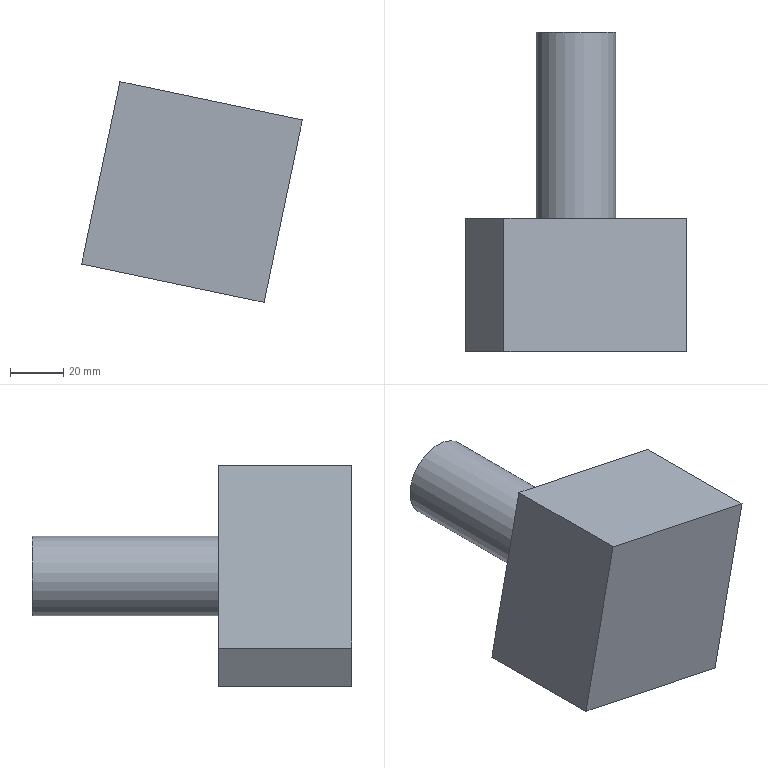Part | STEP file | 5_ESTAGIO_001 | 1 solid | 8 faces | box 82.899 x 120 x 82.899 mm | volume 294480 mm3 | plane 7 | cylinder 1 | commonest cylinder face diameters 30 x1
STEP:
#1=CARTESIAN_POINT('',(0.,0.,0.));
#2=DIRECTION('',(0.,0.,1.));
#3=DIRECTION('',(1.,0.,0.));
#4=AXIS2_PLACEMENT_3D('',#1,#2,#3);
#5=CARTESIAN_POINT('',(-2682.457,-639.15,936.273));
#6=VERTEX_POINT('',#5);
#7=CARTESIAN_POINT('',(-2668.062,-639.15,1004.777));
#8=VERTEX_POINT('',#7);
#9=CARTESIAN_POINT('',(-2682.457,-639.15,936.273));
#10=DIRECTION('',(0.2056,0.,0.9786));
#11=VECTOR('',#10,1.);
#12=LINE('',#9,#11);
#13=CARTESIAN_POINT('',(-2641.008,-639.15,963.327));
#14=DIRECTION('',(0.,1.,0.));
#15=DIRECTION('',(0.,0.,1.));
#16=AXIS2_PLACEMENT_3D('',#13,#14,#15);
#17=PLANE('',#16);
#18=CARTESIAN_POINT('',(-27.054,-41.449));
#19=DIRECTION('',(0.9786,0.2056));
#20=VECTOR('',#19,1.);
#21=LINE('',#18,#20);
#22=(GEOMETRIC_REPRESENTATION_CONTEXT(2)PARAMETRIC_REPRESENTATION_CONTEXT()REPRESENTATION_CONTEXT('',''));
#23=DEFINITIONAL_REPRESENTATION('',(#21),#22);
#24=PCURVE('',#17,#23);
#25=CARTESIAN_POINT('',(-2682.457,-639.15,936.273));
#26=DIRECTION('',(0.9786,0.,-0.2056));
#27=DIRECTION('',(-0.2056,0.,-0.9786));
#28=AXIS2_PLACEMENT_3D('',#25,#26,#27);
#29=PLANE('',#28);
#30=CARTESIAN_POINT('',(-0.000000001,0.));
#31=DIRECTION('',(-1.,0.));
#32=VECTOR('',#31,1.);
#33=LINE('',#30,#32);
#34=(GEOMETRIC_REPRESENTATION_CONTEXT(2)PARAMETRIC_REPRESENTATION_CONTEXT()REPRESENTATION_CONTEXT('',''));
#35=DEFINITIONAL_REPRESENTATION('',(#33),#34);
#36=PCURVE('',#29,#35);
#37=SURFACE_CURVE('',#12,(#24,#36),.PCURVE_S1.);
#38=EDGE_CURVE('',#6,#8,#37,.T.);
#39=ORIENTED_EDGE('',*,*,#38,.T.);
#40=CARTESIAN_POINT('',(-2599.558,-639.15,990.382));
#41=VERTEX_POINT('',#40);
#42=CARTESIAN_POINT('',(-2668.062,-639.15,1004.777));
#43=DIRECTION('',(0.9786,0.,-0.2056));
#44=VECTOR('',#43,1.);
#45=LINE('',#42,#44);
#46=CARTESIAN_POINT('',(41.449,-27.054));
#47=DIRECTION('',(-0.2056,0.9786));
#48=VECTOR('',#47,1.);
#49=LINE('',#46,#48);
#50=(GEOMETRIC_REPRESENTATION_CONTEXT(2)PARAMETRIC_REPRESENTATION_CONTEXT()REPRESENTATION_CONTEXT('',''));
#51=DEFINITIONAL_REPRESENTATION('',(#49),#50);
#52=PCURVE('',#17,#51);
#53=CARTESIAN_POINT('',(-2668.062,-639.15,1004.777));
#54=DIRECTION('',(-0.2056,0.,-0.9786));
#55=DIRECTION('',(-0.9786,0.,0.2056));
#56=AXIS2_PLACEMENT_3D('',#53,#54,#55);
#57=PLANE('',#56);
#58=CARTESIAN_POINT('',(-0.000000002,0.));
#59=DIRECTION('',(-1.,0.));
#60=VECTOR('',#59,1.);
#61=LINE('',#58,#60);
#62=(GEOMETRIC_REPRESENTATION_CONTEXT(2)PARAMETRIC_REPRESENTATION_CONTEXT()REPRESENTATION_CONTEXT('',''));
#63=DEFINITIONAL_REPRESENTATION('',(#61),#62);
#64=PCURVE('',#57,#63);
#65=SURFACE_CURVE('',#45,(#52,#64),.PCURVE_S1.);
#66=EDGE_CURVE('',#8,#41,#65,.T.);
#67=ORIENTED_EDGE('',*,*,#66,.T.);
#68=CARTESIAN_POINT('',(-2613.953,-639.15,921.878));
#69=VERTEX_POINT('',#68);
#70=CARTESIAN_POINT('',(-2599.558,-639.15,990.382));
#71=DIRECTION('',(-0.2056,0.,-0.9786));
#72=VECTOR('',#71,1.);
#73=LINE('',#70,#72);
#74=CARTESIAN_POINT('',(27.054,41.449));
#75=DIRECTION('',(-0.9786,-0.2056));
#76=VECTOR('',#75,1.);
#77=LINE('',#74,#76);
#78=(GEOMETRIC_REPRESENTATION_CONTEXT(2)PARAMETRIC_REPRESENTATION_CONTEXT()REPRESENTATION_CONTEXT('',''));
#79=DEFINITIONAL_REPRESENTATION('',(#77),#78);
#80=PCURVE('',#17,#79);
#81=CARTESIAN_POINT('',(-2599.558,-639.15,990.382));
#82=DIRECTION('',(-0.9786,0.,0.2056));
#83=DIRECTION('',(0.2056,0.,0.9786));
#84=AXIS2_PLACEMENT_3D('',#81,#82,#83);
#85=PLANE('',#84);
#86=CARTESIAN_POINT('',(-0.000000001,0.));
#87=DIRECTION('',(-1.,0.));
#88=VECTOR('',#87,1.);
#89=LINE('',#86,#88);
#90=(GEOMETRIC_REPRESENTATION_CONTEXT(2)PARAMETRIC_REPRESENTATION_CONTEXT()REPRESENTATION_CONTEXT('',''));
#91=DEFINITIONAL_REPRESENTATION('',(#89),#90);
#92=PCURVE('',#85,#91);
#93=SURFACE_CURVE('',#73,(#80,#92),.PCURVE_S1.);
#94=EDGE_CURVE('',#41,#69,#93,.T.);
#95=ORIENTED_EDGE('',*,*,#94,.T.);
#96=CARTESIAN_POINT('',(-2613.953,-639.15,921.878));
#97=DIRECTION('',(-0.9786,0.,0.2056));
#98=VECTOR('',#97,1.);
#99=LINE('',#96,#98);
#100=CARTESIAN_POINT('',(-41.449,27.054));
#101=DIRECTION('',(0.2056,-0.9786));
#102=VECTOR('',#101,1.);
#103=LINE('',#100,#102);
#104=(GEOMETRIC_REPRESENTATION_CONTEXT(2)PARAMETRIC_REPRESENTATION_CONTEXT()REPRESENTATION_CONTEXT('',''));
#105=DEFINITIONAL_REPRESENTATION('',(#103),#104);
#106=PCURVE('',#17,#105);
#107=CARTESIAN_POINT('',(-2613.953,-639.15,921.878));
#108=DIRECTION('',(0.2056,0.,0.9786));
#109=DIRECTION('',(0.9786,0.,-0.2056));
#110=AXIS2_PLACEMENT_3D('',#107,#108,#109);
#111=PLANE('',#110);
#112=CARTESIAN_POINT('',(0.000000002,0.));
#113=DIRECTION('',(-1.,0.));
#114=VECTOR('',#113,1.);
#115=LINE('',#112,#114);
#116=(GEOMETRIC_REPRESENTATION_CONTEXT(2)PARAMETRIC_REPRESENTATION_CONTEXT()REPRESENTATION_CONTEXT('',''));
#117=DEFINITIONAL_REPRESENTATION('',(#115),#116);
#118=PCURVE('',#111,#117);
#119=SURFACE_CURVE('',#99,(#106,#118),.PCURVE_S1.);
#120=EDGE_CURVE('',#69,#6,#119,.T.);
#121=ORIENTED_EDGE('',*,*,#120,.T.);
#122=EDGE_LOOP('',(#39,#67,#95,#121));
#123=FACE_BOUND('',#122,.T.);
#124=CARTESIAN_POINT('',(-2644.092,-639.15,948.648));
#125=VERTEX_POINT('',#124);
#126=CARTESIAN_POINT('',(-2641.008,-639.15,963.327));
#127=DIRECTION('',(0.,1.,0.));
#128=DIRECTION('',(1.,0.,0.));
#129=AXIS2_PLACEMENT_3D('',#126,#127,#128);
#130=CIRCLE('',#129,15.);
#131=CARTESIAN_POINT('',(0.,0.));
#132=DIRECTION('',(0.,1.));
#133=AXIS2_PLACEMENT_2D('',#131,#132);
#134=CIRCLE('',#133,15.);
#135=(GEOMETRIC_REPRESENTATION_CONTEXT(2)PARAMETRIC_REPRESENTATION_CONTEXT()REPRESENTATION_CONTEXT('',''));
#136=DEFINITIONAL_REPRESENTATION('',(#134),#135);
#137=PCURVE('',#17,#136);
#138=CARTESIAN_POINT('',(-2641.008,-604.15,963.327));
#139=DIRECTION('',(0.,1.,0.));
#140=DIRECTION('',(-0.2056,0.,-0.9786));
#141=AXIS2_PLACEMENT_3D('',#138,#139,#140);
#142=CYLINDRICAL_SURFACE('',#141,15.);
#143=CARTESIAN_POINT('',(-1.778,-35.));
#144=DIRECTION('',(1.,0.));
#145=VECTOR('',#144,1.);
#146=LINE('',#143,#145);
#147=(GEOMETRIC_REPRESENTATION_CONTEXT(2)PARAMETRIC_REPRESENTATION_CONTEXT()REPRESENTATION_CONTEXT('',''));
#148=DEFINITIONAL_REPRESENTATION('',(#146),#147);
#149=PCURVE('',#142,#148);
#150=SURFACE_CURVE('',#130,(#137,#149),.PCURVE_S1.);
#151=EDGE_CURVE('',#125,#125,#150,.T.);
#152=ORIENTED_EDGE('',*,*,#151,.F.);
#153=EDGE_LOOP('',(#152));
#154=FACE_BOUND('',#153,.T.);
#155=ADVANCED_FACE('',(#123,#154),#17,.T.);
#156=CARTESIAN_POINT('',(-2613.953,-689.15,921.878));
#157=VERTEX_POINT('',#156);
#158=CARTESIAN_POINT('',(-2682.457,-689.15,936.273));
#159=VERTEX_POINT('',#158);
#160=CARTESIAN_POINT('',(-2613.953,-689.15,921.878));
#161=DIRECTION('',(-0.9786,0.,0.2056));
#162=VECTOR('',#161,1.);
#163=LINE('',#160,#162);
#164=CARTESIAN_POINT('',(0.,-689.15,0.));
#165=DIRECTION('',(0.,-1.,0.));
#166=DIRECTION('',(0.,0.,-1.));
#167=AXIS2_PLACEMENT_3D('',#164,#165,#166);
#168=PLANE('',#167);
#169=CARTESIAN_POINT('',(-921.878,-2613.953));
#170=DIRECTION('',(-0.2056,-0.9786));
#171=VECTOR('',#170,1.);
#172=LINE('',#169,#171);
#173=(GEOMETRIC_REPRESENTATION_CONTEXT(2)PARAMETRIC_REPRESENTATION_CONTEXT()REPRESENTATION_CONTEXT('',''));
#174=DEFINITIONAL_REPRESENTATION('',(#172),#173);
#175=PCURVE('',#168,#174);
#176=CARTESIAN_POINT('',(0.000000002,-50.));
#177=DIRECTION('',(-1.,0.));
#178=VECTOR('',#177,1.);
#179=LINE('',#176,#178);
#180=(GEOMETRIC_REPRESENTATION_CONTEXT(2)PARAMETRIC_REPRESENTATION_CONTEXT()REPRESENTATION_CONTEXT('',''));
#181=DEFINITIONAL_REPRESENTATION('',(#179),#180);
#182=PCURVE('',#111,#181);
#183=SURFACE_CURVE('',#163,(#175,#182),.PCURVE_S1.);
#184=EDGE_CURVE('',#157,#159,#183,.T.);
#185=ORIENTED_EDGE('',*,*,#184,.F.);
#186=CARTESIAN_POINT('',(-2599.558,-689.15,990.382));
#187=VERTEX_POINT('',#186);
#188=CARTESIAN_POINT('',(-2599.558,-689.15,990.382));
#189=DIRECTION('',(-0.2056,0.,-0.9786));
#190=VECTOR('',#189,1.);
#191=LINE('',#188,#190);
#192=CARTESIAN_POINT('',(-990.382,-2599.558));
#193=DIRECTION('',(0.9786,-0.2056));
#194=VECTOR('',#193,1.);
#195=LINE('',#192,#194);
#196=(GEOMETRIC_REPRESENTATION_CONTEXT(2)PARAMETRIC_REPRESENTATION_CONTEXT()REPRESENTATION_CONTEXT('',''));
#197=DEFINITIONAL_REPRESENTATION('',(#195),#196);
#198=PCURVE('',#168,#197);
#199=CARTESIAN_POINT('',(-0.000000001,-50.));
#200=DIRECTION('',(-1.,0.));
#201=VECTOR('',#200,1.);
#202=LINE('',#199,#201);
#203=(GEOMETRIC_REPRESENTATION_CONTEXT(2)PARAMETRIC_REPRESENTATION_CONTEXT()REPRESENTATION_CONTEXT('',''));
#204=DEFINITIONAL_REPRESENTATION('',(#202),#203);
#205=PCURVE('',#85,#204);
#206=SURFACE_CURVE('',#191,(#198,#205),.PCURVE_S1.);
#207=EDGE_CURVE('',#187,#157,#206,.T.);
#208=ORIENTED_EDGE('',*,*,#207,.F.);
#209=CARTESIAN_POINT('',(-2668.062,-689.15,1004.777));
#210=VERTEX_POINT('',#209);
#211=CARTESIAN_POINT('',(-2668.062,-689.15,1004.777));
#212=DIRECTION('',(0.9786,0.,-0.2056));
#213=VECTOR('',#212,1.);
#214=LINE('',#211,#213);
#215=CARTESIAN_POINT('',(-1004.777,-2668.062));
#216=DIRECTION('',(0.2056,0.9786));
#217=VECTOR('',#216,1.);
#218=LINE('',#215,#217);
#219=(GEOMETRIC_REPRESENTATION_CONTEXT(2)PARAMETRIC_REPRESENTATION_CONTEXT()REPRESENTATION_CONTEXT('',''));
#220=DEFINITIONAL_REPRESENTATION('',(#218),#219);
#221=PCURVE('',#168,#220);
#222=CARTESIAN_POINT('',(-0.000000002,-50.));
#223=DIRECTION('',(-1.,0.));
#224=VECTOR('',#223,1.);
#225=LINE('',#222,#224);
#226=(GEOMETRIC_REPRESENTATION_CONTEXT(2)PARAMETRIC_REPRESENTATION_CONTEXT()REPRESENTATION_CONTEXT('',''));
#227=DEFINITIONAL_REPRESENTATION('',(#225),#226);
#228=PCURVE('',#57,#227);
#229=SURFACE_CURVE('',#214,(#221,#228),.PCURVE_S1.);
#230=EDGE_CURVE('',#210,#187,#229,.T.);
#231=ORIENTED_EDGE('',*,*,#230,.F.);
#232=CARTESIAN_POINT('',(-2682.457,-689.15,936.273));
#233=DIRECTION('',(0.2056,0.,0.9786));
#234=VECTOR('',#233,1.);
#235=LINE('',#232,#234);
#236=CARTESIAN_POINT('',(-936.273,-2682.457));
#237=DIRECTION('',(-0.9786,0.2056));
#238=VECTOR('',#237,1.);
#239=LINE('',#236,#238);
#240=(GEOMETRIC_REPRESENTATION_CONTEXT(2)PARAMETRIC_REPRESENTATION_CONTEXT()REPRESENTATION_CONTEXT('',''));
#241=DEFINITIONAL_REPRESENTATION('',(#239),#240);
#242=PCURVE('',#168,#241);
#243=CARTESIAN_POINT('',(-0.000000001,-50.));
#244=DIRECTION('',(-1.,0.));
#245=VECTOR('',#244,1.);
#246=LINE('',#243,#245);
#247=(GEOMETRIC_REPRESENTATION_CONTEXT(2)PARAMETRIC_REPRESENTATION_CONTEXT()REPRESENTATION_CONTEXT('',''));
#248=DEFINITIONAL_REPRESENTATION('',(#246),#247);
#249=PCURVE('',#29,#248);
#250=SURFACE_CURVE('',#235,(#242,#249),.PCURVE_S1.);
#251=EDGE_CURVE('',#159,#210,#250,.T.);
#252=ORIENTED_EDGE('',*,*,#251,.F.);
#253=EDGE_LOOP('',(#185,#208,#231,#252));
#254=FACE_BOUND('',#253,.T.);
#255=ADVANCED_FACE('',(#254),#168,.T.);
#256=CARTESIAN_POINT('',(-2668.062,-639.15,1004.777));
#257=DIRECTION('',(0.,-1.,0.));
#258=VECTOR('',#257,1.);
#259=LINE('',#256,#258);
#260=CARTESIAN_POINT('',(-70.,0.));
#261=DIRECTION('',(0.,-1.));
#262=VECTOR('',#261,1.);
#263=LINE('',#260,#262);
#264=(GEOMETRIC_REPRESENTATION_CONTEXT(2)PARAMETRIC_REPRESENTATION_CONTEXT()REPRESENTATION_CONTEXT('',''));
#265=DEFINITIONAL_REPRESENTATION('',(#263),#264);
#266=PCURVE('',#29,#265);
#267=CARTESIAN_POINT('',(0.,0.));
#268=DIRECTION('',(0.,-1.));
#269=VECTOR('',#268,1.);
#270=LINE('',#267,#269);
#271=(GEOMETRIC_REPRESENTATION_CONTEXT(2)PARAMETRIC_REPRESENTATION_CONTEXT()REPRESENTATION_CONTEXT('',''));
#272=DEFINITIONAL_REPRESENTATION('',(#270),#271);
#273=PCURVE('',#57,#272);
#274=SURFACE_CURVE('',#259,(#266,#273),.PCURVE_S1.);
#275=EDGE_CURVE('',#8,#210,#274,.T.);
#276=ORIENTED_EDGE('',*,*,#275,.F.);
#277=ORIENTED_EDGE('',*,*,#38,.F.);
#278=CARTESIAN_POINT('',(-2682.457,-639.15,936.273));
#279=DIRECTION('',(0.,-1.,0.));
#280=VECTOR('',#279,1.);
#281=LINE('',#278,#280);
#282=CARTESIAN_POINT('',(0.,0.));
#283=DIRECTION('',(0.,-1.));
#284=VECTOR('',#283,1.);
#285=LINE('',#282,#284);
#286=(GEOMETRIC_REPRESENTATION_CONTEXT(2)PARAMETRIC_REPRESENTATION_CONTEXT()REPRESENTATION_CONTEXT('',''));
#287=DEFINITIONAL_REPRESENTATION('',(#285),#286);
#288=PCURVE('',#29,#287);
#289=CARTESIAN_POINT('',(-70.,0.));
#290=DIRECTION('',(0.,-1.));
#291=VECTOR('',#290,1.);
#292=LINE('',#289,#291);
#293=(GEOMETRIC_REPRESENTATION_CONTEXT(2)PARAMETRIC_REPRESENTATION_CONTEXT()REPRESENTATION_CONTEXT('',''));
#294=DEFINITIONAL_REPRESENTATION('',(#292),#293);
#295=PCURVE('',#111,#294);
#296=SURFACE_CURVE('',#281,(#288,#295),.PCURVE_S1.);
#297=EDGE_CURVE('',#6,#159,#296,.T.);
#298=ORIENTED_EDGE('',*,*,#297,.T.);
#299=ORIENTED_EDGE('',*,*,#251,.T.);
#300=EDGE_LOOP('',(#276,#277,#298,#299));
#301=FACE_BOUND('',#300,.T.);
#302=ADVANCED_FACE('',(#301),#29,.F.);
#303=CARTESIAN_POINT('',(-2599.558,-639.15,990.382));
#304=DIRECTION('',(0.,-1.,0.));
#305=VECTOR('',#304,1.);
#306=LINE('',#303,#305);
#307=CARTESIAN_POINT('',(-70.,0.));
#308=DIRECTION('',(0.,-1.));
#309=VECTOR('',#308,1.);
#310=LINE('',#307,#309);
#311=(GEOMETRIC_REPRESENTATION_CONTEXT(2)PARAMETRIC_REPRESENTATION_CONTEXT()REPRESENTATION_CONTEXT('',''));
#312=DEFINITIONAL_REPRESENTATION('',(#310),#311);
#313=PCURVE('',#57,#312);
#314=CARTESIAN_POINT('',(0.,0.));
#315=DIRECTION('',(0.,-1.));
#316=VECTOR('',#315,1.);
#317=LINE('',#314,#316);
#318=(GEOMETRIC_REPRESENTATION_CONTEXT(2)PARAMETRIC_REPRESENTATION_CONTEXT()REPRESENTATION_CONTEXT('',''));
#319=DEFINITIONAL_REPRESENTATION('',(#317),#318);
#320=PCURVE('',#85,#319);
#321=SURFACE_CURVE('',#306,(#313,#320),.PCURVE_S1.);
#322=EDGE_CURVE('',#41,#187,#321,.T.);
#323=ORIENTED_EDGE('',*,*,#322,.F.);
#324=ORIENTED_EDGE('',*,*,#66,.F.);
#325=ORIENTED_EDGE('',*,*,#275,.T.);
#326=ORIENTED_EDGE('',*,*,#230,.T.);
#327=EDGE_LOOP('',(#323,#324,#325,#326));
#328=FACE_BOUND('',#327,.T.);
#329=ADVANCED_FACE('',(#328),#57,.F.);
#330=CARTESIAN_POINT('',(-2613.953,-639.15,921.878));
#331=DIRECTION('',(0.,-1.,0.));
#332=VECTOR('',#331,1.);
#333=LINE('',#330,#332);
#334=CARTESIAN_POINT('',(-70.,0.));
#335=DIRECTION('',(0.,-1.));
#336=VECTOR('',#335,1.);
#337=LINE('',#334,#336);
#338=(GEOMETRIC_REPRESENTATION_CONTEXT(2)PARAMETRIC_REPRESENTATION_CONTEXT()REPRESENTATION_CONTEXT('',''));
#339=DEFINITIONAL_REPRESENTATION('',(#337),#338);
#340=PCURVE('',#85,#339);
#341=CARTESIAN_POINT('',(0.,0.));
#342=DIRECTION('',(0.,-1.));
#343=VECTOR('',#342,1.);
#344=LINE('',#341,#343);
#345=(GEOMETRIC_REPRESENTATION_CONTEXT(2)PARAMETRIC_REPRESENTATION_CONTEXT()REPRESENTATION_CONTEXT('',''));
#346=DEFINITIONAL_REPRESENTATION('',(#344),#345);
#347=PCURVE('',#111,#346);
#348=SURFACE_CURVE('',#333,(#340,#347),.PCURVE_S1.);
#349=EDGE_CURVE('',#69,#157,#348,.T.);
#350=ORIENTED_EDGE('',*,*,#349,.F.);
#351=ORIENTED_EDGE('',*,*,#94,.F.);
#352=ORIENTED_EDGE('',*,*,#322,.T.);
#353=ORIENTED_EDGE('',*,*,#207,.T.);
#354=EDGE_LOOP('',(#350,#351,#352,#353));
#355=FACE_BOUND('',#354,.T.);
#356=ADVANCED_FACE('',(#355),#85,.F.);
#357=ORIENTED_EDGE('',*,*,#297,.F.);
#358=ORIENTED_EDGE('',*,*,#120,.F.);
#359=ORIENTED_EDGE('',*,*,#349,.T.);
#360=ORIENTED_EDGE('',*,*,#184,.T.);
#361=EDGE_LOOP('',(#357,#358,#359,#360));
#362=FACE_BOUND('',#361,.T.);
#363=ADVANCED_FACE('',(#362),#111,.F.);
#364=ORIENTED_EDGE('',*,*,#151,.T.);
#365=CARTESIAN_POINT('',(-2644.092,-569.15,948.648));
#366=VERTEX_POINT('',#365);
#367=CARTESIAN_POINT('',(-2644.092,-639.15,948.648));
#368=CARTESIAN_POINT('',(-2644.092,-569.15,948.648));
#369=B_SPLINE_CURVE_WITH_KNOTS('',1,(#367,#368),.UNSPECIFIED.,.F.,.F.,(2,2),(-35.,35.),.PIECEWISE_BEZIER_KNOTS.);
#370=CARTESIAN_POINT('',(6.283,0.));
#371=DIRECTION('',(0.,1.));
#372=VECTOR('',#371,1.);
#373=LINE('',#370,#372);
#374=(GEOMETRIC_REPRESENTATION_CONTEXT(2)PARAMETRIC_REPRESENTATION_CONTEXT()REPRESENTATION_CONTEXT('',''));
#375=DEFINITIONAL_REPRESENTATION('',(#373),#374);
#376=PCURVE('',#142,#375);
#377=CARTESIAN_POINT('',(0.,0.));
#378=DIRECTION('',(0.,1.));
#379=VECTOR('',#378,1.);
#380=LINE('',#377,#379);
#381=(GEOMETRIC_REPRESENTATION_CONTEXT(2)PARAMETRIC_REPRESENTATION_CONTEXT()REPRESENTATION_CONTEXT('',''));
#382=DEFINITIONAL_REPRESENTATION('',(#380),#381);
#383=PCURVE('',#142,#382);
#384=SEAM_CURVE('',#369,(#376,#383),.PCURVE_S1.);
#385=EDGE_CURVE('',#125,#366,#384,.T.);
#386=ORIENTED_EDGE('',*,*,#385,.T.);
#387=CARTESIAN_POINT('',(-2641.008,-569.15,963.327));
#388=DIRECTION('',(0.,1.,0.));
#389=DIRECTION('',(1.,0.,0.));
#390=AXIS2_PLACEMENT_3D('',#387,#388,#389);
#391=CIRCLE('',#390,15.);
#392=CARTESIAN_POINT('',(-1.778,35.));
#393=DIRECTION('',(1.,0.));
#394=VECTOR('',#393,1.);
#395=LINE('',#392,#394);
#396=(GEOMETRIC_REPRESENTATION_CONTEXT(2)PARAMETRIC_REPRESENTATION_CONTEXT()REPRESENTATION_CONTEXT('',''));
#397=DEFINITIONAL_REPRESENTATION('',(#395),#396);
#398=PCURVE('',#142,#397);
#399=CARTESIAN_POINT('',(-2641.008,-569.15,963.327));
#400=DIRECTION('',(0.,1.,0.));
#401=DIRECTION('',(0.,0.,1.));
#402=AXIS2_PLACEMENT_3D('',#399,#400,#401);
#403=PLANE('',#402);
#404=CARTESIAN_POINT('',(0.,0.));
#405=DIRECTION('',(0.,1.));
#406=AXIS2_PLACEMENT_2D('',#404,#405);
#407=CIRCLE('',#406,15.);
#408=(GEOMETRIC_REPRESENTATION_CONTEXT(2)PARAMETRIC_REPRESENTATION_CONTEXT()REPRESENTATION_CONTEXT('',''));
#409=DEFINITIONAL_REPRESENTATION('',(#407),#408);
#410=PCURVE('',#403,#409);
#411=SURFACE_CURVE('',#391,(#398,#410),.PCURVE_S1.);
#412=EDGE_CURVE('',#366,#366,#411,.T.);
#413=ORIENTED_EDGE('',*,*,#412,.F.);
#414=ORIENTED_EDGE('',*,*,#385,.F.);
#415=EDGE_LOOP('',(#364,#386,#413,#414));
#416=FACE_BOUND('',#415,.T.);
#417=ADVANCED_FACE('',(#416),#142,.T.);
#418=ORIENTED_EDGE('',*,*,#412,.T.);
#419=EDGE_LOOP('',(#418));
#420=FACE_BOUND('',#419,.T.);
#421=ADVANCED_FACE('',(#420),#403,.T.);
#422=CLOSED_SHELL('',(#155,#255,#302,#329,#356,#363,#417,#421));
#423=MANIFOLD_SOLID_BREP('',#422);
#424=(LENGTH_UNIT()NAMED_UNIT(*)SI_UNIT(.MILLI.,.METRE.));
#425=UNCERTAINTY_MEASURE_WITH_UNIT(LENGTH_MEASURE(0.000002),#424,'','');
#426=(NAMED_UNIT(*)PLANE_ANGLE_UNIT()SI_UNIT($,.RADIAN.));
#427=(NAMED_UNIT(*)SI_UNIT($,.STERADIAN.)SOLID_ANGLE_UNIT());
#428=(GEOMETRIC_REPRESENTATION_CONTEXT(3)GLOBAL_UNCERTAINTY_ASSIGNED_CONTEXT((#425))GLOBAL_UNIT_ASSIGNED_CONTEXT((#424,#426,#427))REPRESENTATION_CONTEXT('',''));
#429=ADVANCED_BREP_SHAPE_REPRESENTATION('',(#4,#423),#428);